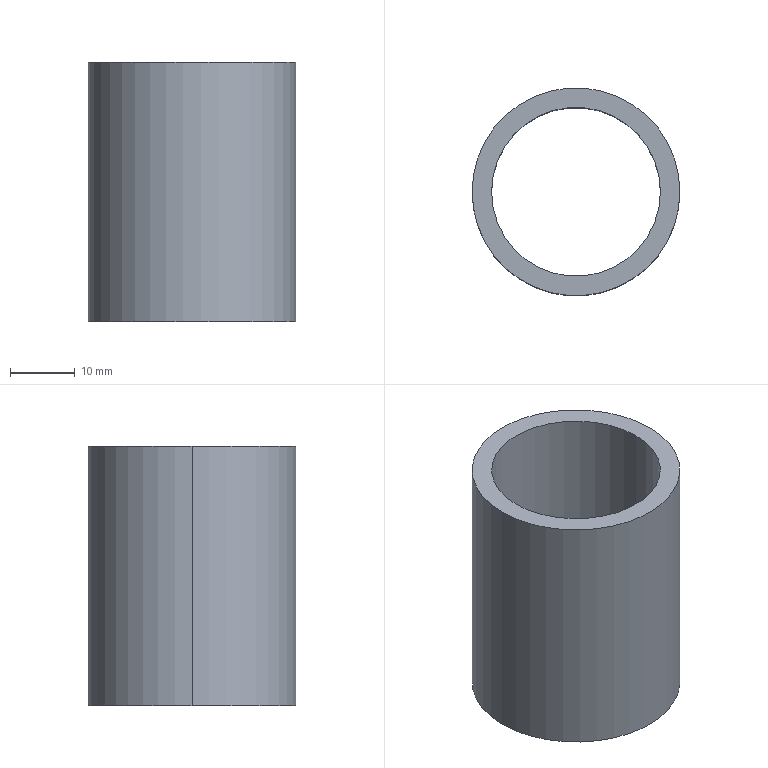Part | SolidWorks | features ExtruThin 1 | 1 solid | 6 faces | box 32 x 32 x 40 mm | volume 10933 mm3 | cylinder 4 | plane 2 | commonest cylinder face diameters 26 x2 32 x2
STEP:
#1=CARTESIAN_POINT('',(-13.,0.,40.));
#2=VERTEX_POINT('',#1);
#3=CARTESIAN_POINT('',(13.,0.,40.));
#4=VERTEX_POINT('',#3);
#5=CARTESIAN_POINT('',(0.,0.,40.));
#6=DIRECTION('',(0.,0.,1.));
#7=DIRECTION('',(1.,0.,0.));
#8=AXIS2_PLACEMENT_3D('',#5,#6,#7);
#9=CIRCLE('',#8,13.);
#10=EDGE_CURVE('',#2,#4,#9,.T.);
#11=ORIENTED_EDGE('',*,*,#10,.T.);
#12=CARTESIAN_POINT('',(13.,0.,0.));
#13=VERTEX_POINT('',#12);
#14=CARTESIAN_POINT('',(13.,0.,40.));
#15=DIRECTION('',(0.,0.,-1.));
#16=VECTOR('',#15,1000.);
#17=LINE('',#14,#16);
#18=EDGE_CURVE('',#4,#13,#17,.T.);
#19=ORIENTED_EDGE('',*,*,#18,.T.);
#20=CARTESIAN_POINT('',(-13.,0.,0.));
#21=VERTEX_POINT('',#20);
#22=CARTESIAN_POINT('',(0.,0.,0.));
#23=DIRECTION('',(0.,0.,1.));
#24=DIRECTION('',(1.,0.,0.));
#25=AXIS2_PLACEMENT_3D('',#22,#23,#24);
#26=CIRCLE('',#25,13.);
#27=EDGE_CURVE('',#21,#13,#26,.T.);
#28=ORIENTED_EDGE('',*,*,#27,.F.);
#29=CARTESIAN_POINT('',(-13.,0.,40.));
#30=DIRECTION('',(0.,0.,-1.));
#31=VECTOR('',#30,1000.);
#32=LINE('',#29,#31);
#33=EDGE_CURVE('',#2,#21,#32,.T.);
#34=ORIENTED_EDGE('',*,*,#33,.F.);
#35=EDGE_LOOP('',(#11,#19,#28,#34));
#36=FACE_OUTER_BOUND('',#35,.T.);
#37=CARTESIAN_POINT('',(0.,0.,40.));
#38=DIRECTION('',(0.,0.,-1.));
#39=DIRECTION('',(-1.,0.,0.));
#40=AXIS2_PLACEMENT_3D('',#37,#38,#39);
#41=CYLINDRICAL_SURFACE('',#40,13.);
#42=ADVANCED_FACE('',(#36),#41,.F.);
#43=CARTESIAN_POINT('',(16.,0.,40.));
#44=VERTEX_POINT('',#43);
#45=CARTESIAN_POINT('',(-16.,0.,40.));
#46=VERTEX_POINT('',#45);
#47=CARTESIAN_POINT('',(0.,0.,40.));
#48=DIRECTION('',(0.,0.,1.));
#49=DIRECTION('',(1.,0.,0.));
#50=AXIS2_PLACEMENT_3D('',#47,#48,#49);
#51=CIRCLE('',#50,16.);
#52=EDGE_CURVE('',#44,#46,#51,.T.);
#53=ORIENTED_EDGE('',*,*,#52,.F.);
#54=CARTESIAN_POINT('',(16.,0.,0.));
#55=VERTEX_POINT('',#54);
#56=CARTESIAN_POINT('',(16.,0.,40.));
#57=DIRECTION('',(0.,0.,-1.));
#58=VECTOR('',#57,1000.);
#59=LINE('',#56,#58);
#60=EDGE_CURVE('',#44,#55,#59,.T.);
#61=ORIENTED_EDGE('',*,*,#60,.T.);
#62=CARTESIAN_POINT('',(-16.,0.,0.));
#63=VERTEX_POINT('',#62);
#64=CARTESIAN_POINT('',(0.,0.,0.));
#65=DIRECTION('',(0.,0.,1.));
#66=DIRECTION('',(1.,0.,0.));
#67=AXIS2_PLACEMENT_3D('',#64,#65,#66);
#68=CIRCLE('',#67,16.);
#69=EDGE_CURVE('',#55,#63,#68,.T.);
#70=ORIENTED_EDGE('',*,*,#69,.T.);
#71=CARTESIAN_POINT('',(-16.,0.,40.));
#72=DIRECTION('',(0.,0.,-1.));
#73=VECTOR('',#72,1000.);
#74=LINE('',#71,#73);
#75=EDGE_CURVE('',#46,#63,#74,.T.);
#76=ORIENTED_EDGE('',*,*,#75,.F.);
#77=EDGE_LOOP('',(#53,#61,#70,#76));
#78=FACE_OUTER_BOUND('',#77,.T.);
#79=CARTESIAN_POINT('',(0.,0.,40.));
#80=DIRECTION('',(0.,0.,-1.));
#81=DIRECTION('',(-1.,0.,0.));
#82=AXIS2_PLACEMENT_3D('',#79,#80,#81);
#83=CYLINDRICAL_SURFACE('',#82,16.);
#84=ADVANCED_FACE('',(#78),#83,.T.);
#85=CARTESIAN_POINT('',(0.,0.,40.));
#86=DIRECTION('',(0.,0.,1.));
#87=DIRECTION('',(1.,0.,0.));
#88=AXIS2_PLACEMENT_3D('',#85,#86,#87);
#89=CIRCLE('',#88,16.);
#90=EDGE_CURVE('',#46,#44,#89,.T.);
#91=ORIENTED_EDGE('',*,*,#90,.T.);
#92=ORIENTED_EDGE('',*,*,#52,.T.);
#93=EDGE_LOOP('',(#91,#92));
#94=FACE_OUTER_BOUND('',#93,.T.);
#95=ORIENTED_EDGE('',*,*,#10,.F.);
#96=CARTESIAN_POINT('',(0.,0.,40.));
#97=DIRECTION('',(0.,0.,1.));
#98=DIRECTION('',(1.,0.,0.));
#99=AXIS2_PLACEMENT_3D('',#96,#97,#98);
#100=CIRCLE('',#99,13.);
#101=EDGE_CURVE('',#4,#2,#100,.T.);
#102=ORIENTED_EDGE('',*,*,#101,.F.);
#103=EDGE_LOOP('',(#95,#102));
#104=FACE_BOUND('',#103,.T.);
#105=CARTESIAN_POINT('',(0.,0.,40.));
#106=DIRECTION('',(0.,0.,1.));
#107=DIRECTION('',(1.,0.,0.));
#108=AXIS2_PLACEMENT_3D('',#105,#106,#107);
#109=PLANE('',#108);
#110=ADVANCED_FACE('',(#94,#104),#109,.T.);
#111=CARTESIAN_POINT('',(0.,0.,0.));
#112=DIRECTION('',(0.,0.,1.));
#113=DIRECTION('',(1.,0.,0.));
#114=AXIS2_PLACEMENT_3D('',#111,#112,#113);
#115=CIRCLE('',#114,16.);
#116=EDGE_CURVE('',#63,#55,#115,.T.);
#117=ORIENTED_EDGE('',*,*,#116,.F.);
#118=ORIENTED_EDGE('',*,*,#69,.F.);
#119=EDGE_LOOP('',(#117,#118));
#120=FACE_OUTER_BOUND('',#119,.T.);
#121=ORIENTED_EDGE('',*,*,#27,.T.);
#122=CARTESIAN_POINT('',(0.,0.,0.));
#123=DIRECTION('',(0.,0.,1.));
#124=DIRECTION('',(1.,0.,0.));
#125=AXIS2_PLACEMENT_3D('',#122,#123,#124);
#126=CIRCLE('',#125,13.);
#127=EDGE_CURVE('',#13,#21,#126,.T.);
#128=ORIENTED_EDGE('',*,*,#127,.T.);
#129=EDGE_LOOP('',(#121,#128));
#130=FACE_BOUND('',#129,.T.);
#131=CARTESIAN_POINT('',(0.,0.,0.));
#132=DIRECTION('',(0.,0.,1.));
#133=DIRECTION('',(1.,0.,0.));
#134=AXIS2_PLACEMENT_3D('',#131,#132,#133);
#135=PLANE('',#134);
#136=ADVANCED_FACE('',(#120,#130),#135,.F.);
#137=ORIENTED_EDGE('',*,*,#60,.F.);
#138=ORIENTED_EDGE('',*,*,#90,.F.);
#139=ORIENTED_EDGE('',*,*,#75,.T.);
#140=ORIENTED_EDGE('',*,*,#116,.T.);
#141=EDGE_LOOP('',(#137,#138,#139,#140));
#142=FACE_OUTER_BOUND('',#141,.T.);
#143=CARTESIAN_POINT('',(0.,0.,40.));
#144=DIRECTION('',(0.,0.,-1.));
#145=DIRECTION('',(-1.,0.,0.));
#146=AXIS2_PLACEMENT_3D('',#143,#144,#145);
#147=CYLINDRICAL_SURFACE('',#146,16.);
#148=ADVANCED_FACE('',(#142),#147,.T.);
#149=ORIENTED_EDGE('',*,*,#18,.F.);
#150=ORIENTED_EDGE('',*,*,#101,.T.);
#151=ORIENTED_EDGE('',*,*,#33,.T.);
#152=ORIENTED_EDGE('',*,*,#127,.F.);
#153=EDGE_LOOP('',(#149,#150,#151,#152));
#154=FACE_OUTER_BOUND('',#153,.T.);
#155=CARTESIAN_POINT('',(0.,0.,40.));
#156=DIRECTION('',(0.,0.,-1.));
#157=DIRECTION('',(-1.,0.,0.));
#158=AXIS2_PLACEMENT_3D('',#155,#156,#157);
#159=CYLINDRICAL_SURFACE('',#158,13.);
#160=ADVANCED_FACE('',(#154),#159,.F.);
#161=CLOSED_SHELL('',(#42,#84,#110,#136,#148,#160));
#162=MANIFOLD_SOLID_BREP('',#161);
#163=CARTESIAN_POINT('',(0.,0.,0.));
#164=DIRECTION('',(0.,0.,1.));
#165=DIRECTION('',(1.,0.,0.));
#166=AXIS2_PLACEMENT_3D('',#163,#164,#165);
#167=(LENGTH_UNIT()NAMED_UNIT(*)SI_UNIT(.MILLI.,.METRE.));
#168=UNCERTAINTY_MEASURE_WITH_UNIT(LENGTH_MEASURE(0.00001),#167,'','');
#169=(NAMED_UNIT(*)PLANE_ANGLE_UNIT()SI_UNIT($,.RADIAN.));
#170=(NAMED_UNIT(*)SI_UNIT($,.STERADIAN.)SOLID_ANGLE_UNIT());
#171=(GEOMETRIC_REPRESENTATION_CONTEXT(3)GLOBAL_UNCERTAINTY_ASSIGNED_CONTEXT((#168))GLOBAL_UNIT_ASSIGNED_CONTEXT((#167,#169,#170))REPRESENTATION_CONTEXT('',''));
#172=ADVANCED_BREP_SHAPE_REPRESENTATION('',(#162,#166),#171);